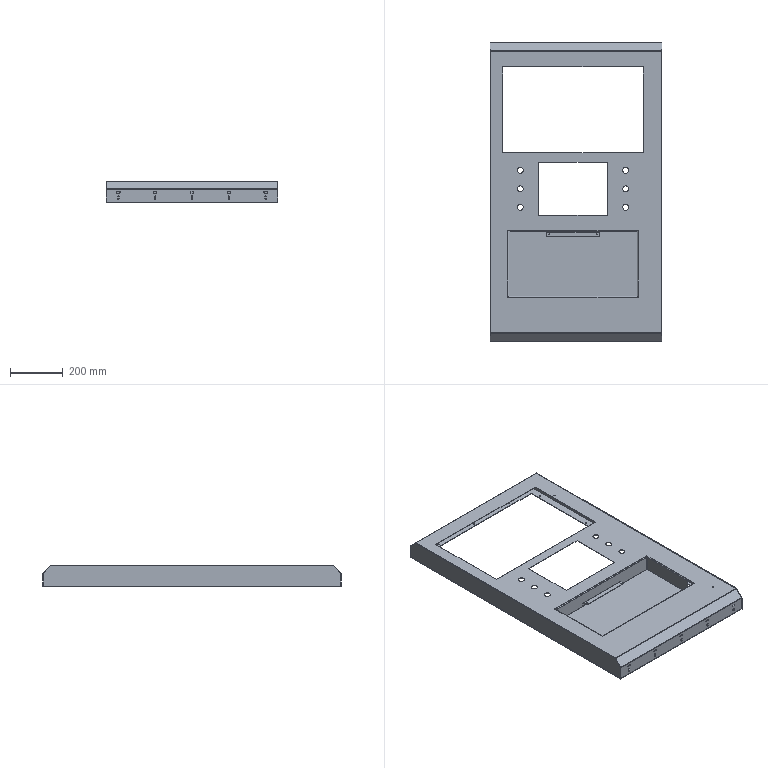Part | NX | features BREP 6 | 6 solids | 275 faces | box 650 x 1132 x 82 mm | volume 1596159 mm3 | plane 138 | cylinder 129 | spline 8 | commonest cylinder face diameters 4.2 x40 6 x37 4 x19 22.5 x12 7 x8 16 x6